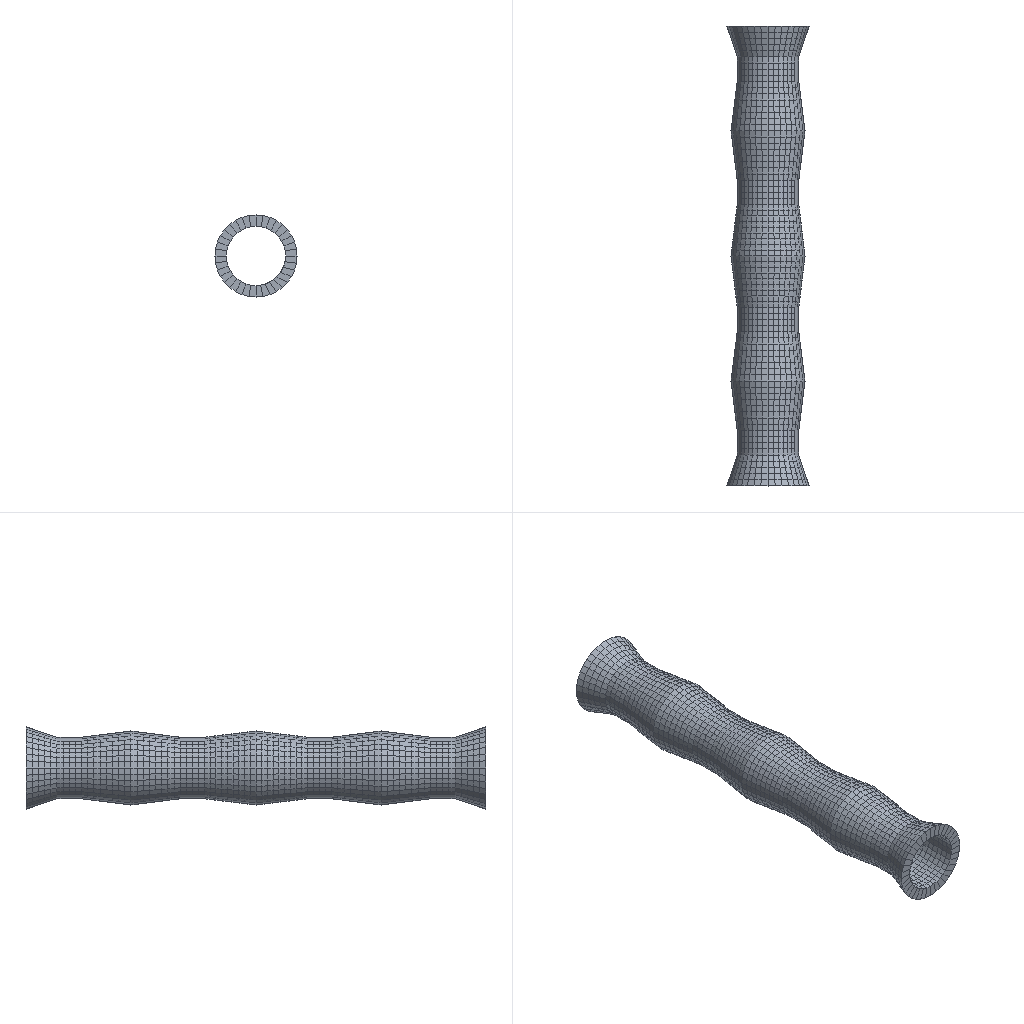Simulation study | abaqus
Set-up summary:
category,name,step,type,value,unit,region
solver,abaqus
solver,version,,,Abaqus/Standard 2020
units,not stated in the deck,,not stated
analysis,deck,,static,static
load_step,Step-1,Step-1,static
load_step,requested,,,1
mesh,nodes,,,5544
mesh,elements,,,2736
element_type,C3D8R,,solid,2736
load,load commands in deck,,count,1
bc,support commands in deck,,count,1
material,MATERIAL-1,,in results
check,setup vs results,,match,"per instance, exact: element labels, types and connectivity; labels of the nodes the elements use; coordinates of those nodes at SINGLE_PRECISION in 1 of 1 instance(s)"
Abaqus input file, long lists of numbers shortened:
*Heading
** Job name: Job-1 Model name: Model-1
** Generated by: Abaqus/CAE 2020
*Preprint, echo=NO, model=NO, history=NO, contact=NO
**
** PARTS
**
*Part, name=final
*Node
      1,         -75.,       -187.5,           0.
      2,         -60.,       -187.5,           0.
** (5542 more lines like these left out)
*Element, type=C3D8R
 1,  160,  168, 1505, 1449,    1,    2,  115,  130
 2, 1449, 1505, 1506, 1450,  130,  115,  116,  129
** (2734 more lines like these left out)
*Nset, nset=Set-1, generate
    1,  5544,     1
*Elset, elset=Set-1, generate
    1,  2736,     1
** Section: Section-1
*Solid Section, elset=Set-1, material=Material-1
,
*End Part
**
**
** ASSEMBLY
**
*Assembly, name=Assembly
**
*Instance, name=final-1, part=final
*End Instance
**
*Nset, nset=Set-1, instance=final-1
    7,    8,   12,   17,   20,   21,   23,   26,   27,   30,   36,   39,   44,   47,   49,   50
   59,   60,   64,   69,   72,   73,   75,   78,   80,   83,   88,   89,   92,   96,  101,  104
** (43 more lines like these left out)
*Elset, elset=Set-1, instance=final-1
 1621, 1622, 1623, 1624, 1625, 1626, 1627, 1628, 1629, 1630, 1631, 1632, 1633, 1634, 1635, 1636
 1637, 1638, 1639, 1640, 1641, 1642, 1643, 1644, 1645, 1646, 1647, 1648, 1649, 1650, 1651, 1652
** (34 more lines like these left out)
*Elset, elset=_Surf-1_S6, internal, instance=final-1
  586,  587,  588,  589,  590,  591,  592,  593,  594,  595,  596,  597,  598,  599,  600,  601
  602,  603,  604,  605,  606,  607,  608,  609,  610,  611,  612,  613,  614,  615,  616,  617
** (62 more lines like these left out)
*Elset, elset=_Surf-1_S4, internal, instance=final-1
    1,    2,    3,    4,    5,    6,    7,    8,    9,   10,   11,   12,   13,   14,   15,   16
   17,   18,   19,   20,   21,   22,   23,   24,   25,   26,   27,   28,   29,   30,   31,   32
** (82 more lines like these left out)
*Elset, elset=_Surf-1_S5, internal, instance=final-1
  145,  146,  147,  148,  149,  150,  151,  152,  153,  154,  155,  156,  157,  158,  159,  160
  161,  162,  163,  164,  165,  166,  167,  168,  169,  170,  171,  172,  173,  174,  175,  176
** (16 more lines like these left out)
*Elset, elset=_Surf-1_S1, internal, instance=final-1
 2179, 2180, 2181, 2182, 2183, 2184, 2185, 2186, 2187, 2188, 2189, 2190, 2191, 2192, 2193, 2194
 2195, 2196, 2197, 2198, 2199, 2200, 2201, 2202, 2203, 2204, 2205, 2206, 2207, 2208, 2209, 2210
** (4 more lines like these left out)
*Surface, type=ELEMENT, name=Surf-1
_Surf-1_S6, S6
_Surf-1_S4, S4
_Surf-1_S5, S5
_Surf-1_S1, S1
*End Assembly
*Amplitude, name=Amp-1
             0.,              0.,              1.,              1.
**
** MATERIALS
**
*Material, name=Material-1
*Density
 7.8e-09,
*Elastic
210000., 0.3
*Plastic
450.,0.
** ----------------------------------------------------------------
**
** STEP: Step-1
**
*Step, name=Step-1, nlgeom=YES, inc=1000
*Static, stabilize=0.0002, allsdtol=0.05, continue=NO
0.01, 1., 1e-05, 1.
**
** BOUNDARY CONDITIONS
**
** Name: BC-1 Type: 对称/反对称/完全固定
*Boundary
Set-1, ENCASTRE
**
** LOADS
**
** Name: Load-1   Type: Pressure
*Dsload, amplitude=Amp-1
Surf-1, P, 50.
**
** OUTPUT REQUESTS
**
*Restart, write, frequency=0
**
** FIELD OUTPUT: F-Output-1
**
*Output, field, variable=PRESELECT
**
** HISTORY OUTPUT: H-Output-1
**
*Output, history, variable=PRESELECT
*End Step
Results summary:
result,step,,completed,increments=11 time=1.0/1.0
result,analysis,,,static
result,last_loadstep,,,1
result,primary field,,,U
result,reaction total,,FX,-7.103,model units
result,reaction total,,FY,-0.02731,model units
result,reaction total,,FZ,-5.176,model units